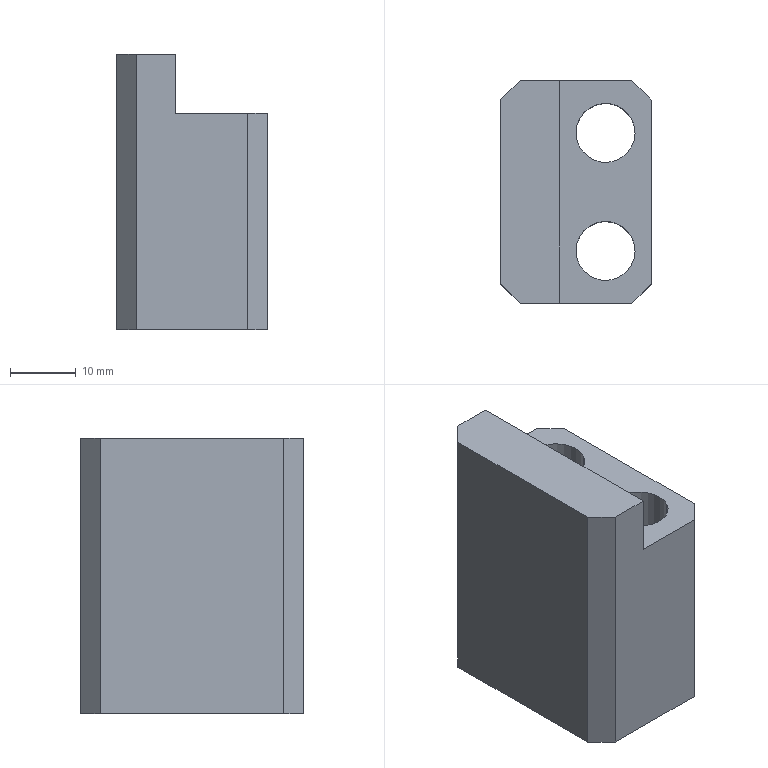Part | CATIA | 1 solid | 16 faces | box 23 x 34 x 42 mm | volume 23686 mm3 | plane 12 | cylinder 4 | commonest cylinder face diameters 9 x4
STEP:
#1=CARTESIAN_POINT('',(-1248.,-1169.,-42.));
#2=VERTEX_POINT('',#1);
#3=CARTESIAN_POINT('',(-1245.,-1172.,-42.));
#4=VERTEX_POINT('',#3);
#5=CARTESIAN_POINT('',(-1246.5,-1170.5,-42.));
#6=DIRECTION('',(0.7071,-0.7071,0.));
#7=VECTOR('',#6,1.);
#8=LINE('',#5,#7);
#9=EDGE_CURVE('',#2,#4,#8,.T.);
#10=ORIENTED_EDGE('',*,*,#9,.T.);
#11=CARTESIAN_POINT('',(-1245.,-1172.,0.));
#12=VERTEX_POINT('',#11);
#13=CARTESIAN_POINT('',(-1245.,-1172.,-21.));
#14=DIRECTION('',(0.,0.,-1.));
#15=VECTOR('',#14,1.);
#16=LINE('',#13,#15);
#17=EDGE_CURVE('',#12,#4,#16,.T.);
#18=ORIENTED_EDGE('',*,*,#17,.F.);
#19=CARTESIAN_POINT('',(-1248.,-1169.,0.));
#20=VERTEX_POINT('',#19);
#21=CARTESIAN_POINT('',(-1246.5,-1170.5,0.));
#22=DIRECTION('',(0.7071,-0.7071,0.));
#23=VECTOR('',#22,1.);
#24=LINE('',#21,#23);
#25=EDGE_CURVE('',#12,#20,#24,.F.);
#26=ORIENTED_EDGE('',*,*,#25,.T.);
#27=CARTESIAN_POINT('',(-1248.,-1169.,-21.));
#28=DIRECTION('',(0.,0.,-1.));
#29=VECTOR('',#28,1.);
#30=LINE('',#27,#29);
#31=EDGE_CURVE('',#20,#2,#30,.T.);
#32=ORIENTED_EDGE('',*,*,#31,.T.);
#33=EDGE_LOOP('',(#10,#18,#26,#32));
#34=FACE_OUTER_BOUND('',#33,.T.);
#35=CARTESIAN_POINT('',(-1248.,-1169.,8.4));
#36=DIRECTION('',(-0.7071,-0.7071,0.));
#37=DIRECTION('',(0.,0.,-1.));
#38=AXIS2_PLACEMENT_3D('',#35,#36,#37);
#39=PLANE('',#38);
#40=ADVANCED_FACE('',(#34),#39,.T.);
#41=CARTESIAN_POINT('',(-1248.,-1141.,0.));
#42=VERTEX_POINT('',#41);
#43=CARTESIAN_POINT('',(-1248.,-1141.,-42.));
#44=VERTEX_POINT('',#43);
#45=CARTESIAN_POINT('',(-1248.,-1141.,-21.));
#46=DIRECTION('',(0.,0.,1.));
#47=VECTOR('',#46,1.);
#48=LINE('',#45,#47);
#49=EDGE_CURVE('',#42,#44,#48,.F.);
#50=ORIENTED_EDGE('',*,*,#49,.T.);
#51=CARTESIAN_POINT('',(-1248.,-1155.,-42.));
#52=DIRECTION('',(0.,-1.,0.));
#53=VECTOR('',#52,1.);
#54=LINE('',#51,#53);
#55=EDGE_CURVE('',#44,#2,#54,.T.);
#56=ORIENTED_EDGE('',*,*,#55,.T.);
#57=ORIENTED_EDGE('',*,*,#31,.F.);
#58=CARTESIAN_POINT('',(-1248.,-1155.,0.));
#59=DIRECTION('',(0.,-1.,0.));
#60=VECTOR('',#59,1.);
#61=LINE('',#58,#60);
#62=EDGE_CURVE('',#42,#20,#61,.T.);
#63=ORIENTED_EDGE('',*,*,#62,.F.);
#64=EDGE_LOOP('',(#50,#56,#57,#63));
#65=FACE_OUTER_BOUND('',#64,.T.);
#66=CARTESIAN_POINT('',(-1248.,-1138.,0.));
#67=DIRECTION('',(1.,0.,0.));
#68=DIRECTION('',(0.,-1.,0.));
#69=AXIS2_PLACEMENT_3D('',#66,#67,#68);
#70=PLANE('',#69);
#71=ADVANCED_FACE('',(#65),#70,.F.);
#72=CARTESIAN_POINT('',(-1245.,-1138.,-42.));
#73=VERTEX_POINT('',#72);
#74=CARTESIAN_POINT('',(-1246.5,-1139.5,-42.));
#75=DIRECTION('',(0.7071,0.7071,0.));
#76=VECTOR('',#75,1.);
#77=LINE('',#74,#76);
#78=EDGE_CURVE('',#73,#44,#77,.F.);
#79=ORIENTED_EDGE('',*,*,#78,.T.);
#80=ORIENTED_EDGE('',*,*,#49,.F.);
#81=CARTESIAN_POINT('',(-1245.,-1138.,0.));
#82=VERTEX_POINT('',#81);
#83=CARTESIAN_POINT('',(-1246.5,-1139.5,0.));
#84=DIRECTION('',(0.7071,0.7071,0.));
#85=VECTOR('',#84,1.);
#86=LINE('',#83,#85);
#87=EDGE_CURVE('',#42,#82,#86,.T.);
#88=ORIENTED_EDGE('',*,*,#87,.T.);
#89=CARTESIAN_POINT('',(-1245.,-1138.,-21.));
#90=DIRECTION('',(0.,0.,1.));
#91=VECTOR('',#90,1.);
#92=LINE('',#89,#91);
#93=EDGE_CURVE('',#82,#73,#92,.F.);
#94=ORIENTED_EDGE('',*,*,#93,.T.);
#95=EDGE_LOOP('',(#79,#80,#88,#94));
#96=FACE_OUTER_BOUND('',#95,.T.);
#97=CARTESIAN_POINT('',(-1248.,-1141.,-50.4));
#98=DIRECTION('',(-0.7071,0.7071,0.));
#99=DIRECTION('',(0.,0.,1.));
#100=AXIS2_PLACEMENT_3D('',#97,#98,#99);
#101=PLANE('',#100);
#102=ADVANCED_FACE('',(#96),#101,.T.);
#103=CARTESIAN_POINT('',(-1225.,-1141.,-9.));
#104=VERTEX_POINT('',#103);
#105=CARTESIAN_POINT('',(-1225.,-1141.,-42.));
#106=VERTEX_POINT('',#105);
#107=CARTESIAN_POINT('',(-1225.,-1141.,-21.));
#108=DIRECTION('',(0.,0.,-1.));
#109=VECTOR('',#108,1.);
#110=LINE('',#107,#109);
#111=EDGE_CURVE('',#104,#106,#110,.T.);
#112=ORIENTED_EDGE('',*,*,#111,.T.);
#113=CARTESIAN_POINT('',(-1228.,-1138.,-42.));
#114=VERTEX_POINT('',#113);
#115=CARTESIAN_POINT('',(-1226.5,-1139.5,-42.));
#116=DIRECTION('',(-0.7071,0.7071,0.));
#117=VECTOR('',#116,1.);
#118=LINE('',#115,#117);
#119=EDGE_CURVE('',#106,#114,#118,.T.);
#120=ORIENTED_EDGE('',*,*,#119,.T.);
#121=CARTESIAN_POINT('',(-1228.,-1138.,-9.));
#122=VERTEX_POINT('',#121);
#123=CARTESIAN_POINT('',(-1228.,-1138.,-21.));
#124=DIRECTION('',(0.,0.,-1.));
#125=VECTOR('',#124,1.);
#126=LINE('',#123,#125);
#127=EDGE_CURVE('',#122,#114,#126,.T.);
#128=ORIENTED_EDGE('',*,*,#127,.F.);
#129=CARTESIAN_POINT('',(-1226.5,-1139.5,-9.));
#130=DIRECTION('',(-0.7071,0.7071,0.));
#131=VECTOR('',#130,1.);
#132=LINE('',#129,#131);
#133=EDGE_CURVE('',#122,#104,#132,.F.);
#134=ORIENTED_EDGE('',*,*,#133,.T.);
#135=EDGE_LOOP('',(#112,#120,#128,#134));
#136=FACE_OUTER_BOUND('',#135,.T.);
#137=CARTESIAN_POINT('',(-1225.,-1141.,8.4));
#138=DIRECTION('',(0.7071,0.7071,0.));
#139=DIRECTION('',(0.,0.,-1.));
#140=AXIS2_PLACEMENT_3D('',#137,#138,#139);
#141=PLANE('',#140);
#142=ADVANCED_FACE('',(#136),#141,.T.);
#143=CARTESIAN_POINT('',(-1239.,-1138.,0.));
#144=VERTEX_POINT('',#143);
#145=CARTESIAN_POINT('',(-1242.,-1138.,0.));
#146=DIRECTION('',(1.,0.,0.));
#147=VECTOR('',#146,1.);
#148=LINE('',#145,#147);
#149=EDGE_CURVE('',#144,#82,#148,.F.);
#150=ORIENTED_EDGE('',*,*,#149,.T.);
#151=ORIENTED_EDGE('',*,*,#87,.F.);
#152=ORIENTED_EDGE('',*,*,#62,.T.);
#153=ORIENTED_EDGE('',*,*,#25,.F.);
#154=CARTESIAN_POINT('',(-1239.,-1172.,0.));
#155=VERTEX_POINT('',#154);
#156=CARTESIAN_POINT('',(-1242.,-1172.,0.));
#157=DIRECTION('',(-1.,0.,0.));
#158=VECTOR('',#157,1.);
#159=LINE('',#156,#158);
#160=EDGE_CURVE('',#12,#155,#159,.F.);
#161=ORIENTED_EDGE('',*,*,#160,.T.);
#162=CARTESIAN_POINT('',(-1239.,-1155.,0.));
#163=DIRECTION('',(0.,-1.,0.));
#164=VECTOR('',#163,1.);
#165=LINE('',#162,#164);
#166=EDGE_CURVE('',#144,#155,#165,.T.);
#167=ORIENTED_EDGE('',*,*,#166,.F.);
#168=EDGE_LOOP('',(#150,#151,#152,#153,#161,#167));
#169=FACE_OUTER_BOUND('',#168,.T.);
#170=CARTESIAN_POINT('',(0.,0.,0.));
#171=DIRECTION('',(0.,0.,1.));
#172=DIRECTION('',(1.,0.,0.));
#173=AXIS2_PLACEMENT_3D('',#170,#171,#172);
#174=PLANE('',#173);
#175=ADVANCED_FACE('',(#169),#174,.T.);
#176=CARTESIAN_POINT('',(-1225.,-1169.,-9.));
#177=VERTEX_POINT('',#176);
#178=CARTESIAN_POINT('',(-1225.,-1155.,-9.));
#179=DIRECTION('',(0.,1.,0.));
#180=VECTOR('',#179,1.);
#181=LINE('',#178,#180);
#182=EDGE_CURVE('',#177,#104,#181,.T.);
#183=ORIENTED_EDGE('',*,*,#182,.F.);
#184=CARTESIAN_POINT('',(-1225.,-1169.,-42.));
#185=VERTEX_POINT('',#184);
#186=CARTESIAN_POINT('',(-1225.,-1169.,-25.5));
#187=DIRECTION('',(0.,0.,1.));
#188=VECTOR('',#187,1.);
#189=LINE('',#186,#188);
#190=EDGE_CURVE('',#177,#185,#189,.F.);
#191=ORIENTED_EDGE('',*,*,#190,.T.);
#192=CARTESIAN_POINT('',(-1225.,-1155.,-42.));
#193=DIRECTION('',(0.,1.,0.));
#194=VECTOR('',#193,1.);
#195=LINE('',#192,#194);
#196=EDGE_CURVE('',#185,#106,#195,.T.);
#197=ORIENTED_EDGE('',*,*,#196,.T.);
#198=ORIENTED_EDGE('',*,*,#111,.F.);
#199=EDGE_LOOP('',(#183,#191,#197,#198));
#200=FACE_OUTER_BOUND('',#199,.T.);
#201=CARTESIAN_POINT('',(-1225.,-1172.,0.));
#202=DIRECTION('',(-1.,0.,0.));
#203=DIRECTION('',(0.,1.,0.));
#204=AXIS2_PLACEMENT_3D('',#201,#202,#203);
#205=PLANE('',#204);
#206=ADVANCED_FACE('',(#200),#205,.F.);
#207=ORIENTED_EDGE('',*,*,#127,.T.);
#208=CARTESIAN_POINT('',(-1236.5,-1138.,-42.));
#209=DIRECTION('',(1.,0.,0.));
#210=VECTOR('',#209,1.);
#211=LINE('',#208,#210);
#212=EDGE_CURVE('',#73,#114,#211,.T.);
#213=ORIENTED_EDGE('',*,*,#212,.F.);
#214=ORIENTED_EDGE('',*,*,#93,.F.);
#215=ORIENTED_EDGE('',*,*,#149,.F.);
#216=CARTESIAN_POINT('',(-1239.,-1138.,-9.));
#217=VERTEX_POINT('',#216);
#218=CARTESIAN_POINT('',(-1239.,-1138.,-4.5));
#219=DIRECTION('',(0.,0.,1.));
#220=VECTOR('',#219,1.);
#221=LINE('',#218,#220);
#222=EDGE_CURVE('',#217,#144,#221,.T.);
#223=ORIENTED_EDGE('',*,*,#222,.F.);
#224=CARTESIAN_POINT('',(-1233.5,-1138.,-9.));
#225=DIRECTION('',(1.,0.,0.));
#226=VECTOR('',#225,1.);
#227=LINE('',#224,#226);
#228=EDGE_CURVE('',#217,#122,#227,.T.);
#229=ORIENTED_EDGE('',*,*,#228,.T.);
#230=EDGE_LOOP('',(#207,#213,#214,#215,#223,#229));
#231=FACE_OUTER_BOUND('',#230,.T.);
#232=CARTESIAN_POINT('',(-1248.,-1138.,0.));
#233=DIRECTION('',(0.,1.,0.));
#234=DIRECTION('',(1.,0.,0.));
#235=AXIS2_PLACEMENT_3D('',#232,#233,#234);
#236=PLANE('',#235);
#237=ADVANCED_FACE('',(#231),#236,.T.);
#238=CARTESIAN_POINT('',(-1228.,-1172.,-9.));
#239=VERTEX_POINT('',#238);
#240=CARTESIAN_POINT('',(-1228.,-1172.,-42.));
#241=VERTEX_POINT('',#240);
#242=CARTESIAN_POINT('',(-1228.,-1172.,-21.));
#243=DIRECTION('',(0.,0.,1.));
#244=VECTOR('',#243,1.);
#245=LINE('',#242,#244);
#246=EDGE_CURVE('',#239,#241,#245,.F.);
#247=ORIENTED_EDGE('',*,*,#246,.T.);
#248=CARTESIAN_POINT('',(-1226.5,-1170.5,-42.));
#249=DIRECTION('',(-0.7071,-0.7071,0.));
#250=VECTOR('',#249,1.);
#251=LINE('',#248,#250);
#252=EDGE_CURVE('',#241,#185,#251,.F.);
#253=ORIENTED_EDGE('',*,*,#252,.T.);
#254=ORIENTED_EDGE('',*,*,#190,.F.);
#255=CARTESIAN_POINT('',(-1226.5,-1170.5,-9.));
#256=DIRECTION('',(-0.7071,-0.7071,0.));
#257=VECTOR('',#256,1.);
#258=LINE('',#255,#257);
#259=EDGE_CURVE('',#239,#177,#258,.F.);
#260=ORIENTED_EDGE('',*,*,#259,.F.);
#261=EDGE_LOOP('',(#247,#253,#254,#260));
#262=FACE_OUTER_BOUND('',#261,.T.);
#263=CARTESIAN_POINT('',(-1225.,-1169.,-50.4));
#264=DIRECTION('',(0.7071,-0.7071,0.));
#265=DIRECTION('',(0.,0.,1.));
#266=AXIS2_PLACEMENT_3D('',#263,#264,#265);
#267=PLANE('',#266);
#268=ADVANCED_FACE('',(#262),#267,.T.);
#269=ORIENTED_EDGE('',*,*,#160,.F.);
#270=ORIENTED_EDGE('',*,*,#17,.T.);
#271=CARTESIAN_POINT('',(-1236.5,-1172.,-42.));
#272=DIRECTION('',(-1.,0.,0.));
#273=VECTOR('',#272,1.);
#274=LINE('',#271,#273);
#275=EDGE_CURVE('',#241,#4,#274,.T.);
#276=ORIENTED_EDGE('',*,*,#275,.F.);
#277=ORIENTED_EDGE('',*,*,#246,.F.);
#278=CARTESIAN_POINT('',(-1239.,-1172.,-9.));
#279=VERTEX_POINT('',#278);
#280=CARTESIAN_POINT('',(-1233.5,-1172.,-9.));
#281=DIRECTION('',(1.,0.,0.));
#282=VECTOR('',#281,1.);
#283=LINE('',#280,#282);
#284=EDGE_CURVE('',#279,#239,#283,.T.);
#285=ORIENTED_EDGE('',*,*,#284,.F.);
#286=CARTESIAN_POINT('',(-1239.,-1172.,-4.5));
#287=DIRECTION('',(0.,0.,1.));
#288=VECTOR('',#287,1.);
#289=LINE('',#286,#288);
#290=EDGE_CURVE('',#279,#155,#289,.T.);
#291=ORIENTED_EDGE('',*,*,#290,.T.);
#292=EDGE_LOOP('',(#269,#270,#276,#277,#285,#291));
#293=FACE_OUTER_BOUND('',#292,.T.);
#294=CARTESIAN_POINT('',(-1225.,-1172.,0.));
#295=DIRECTION('',(0.,-1.,0.));
#296=DIRECTION('',(-1.,0.,0.));
#297=AXIS2_PLACEMENT_3D('',#294,#295,#296);
#298=PLANE('',#297);
#299=ADVANCED_FACE('',(#293),#298,.T.);
#300=CARTESIAN_POINT('',(-1239.,-1155.,-9.));
#301=DIRECTION('',(0.,-1.,0.));
#302=VECTOR('',#301,1.);
#303=LINE('',#300,#302);
#304=EDGE_CURVE('',#217,#279,#303,.T.);
#305=ORIENTED_EDGE('',*,*,#304,.F.);
#306=ORIENTED_EDGE('',*,*,#222,.T.);
#307=ORIENTED_EDGE('',*,*,#166,.T.);
#308=ORIENTED_EDGE('',*,*,#290,.F.);
#309=EDGE_LOOP('',(#305,#306,#307,#308));
#310=FACE_OUTER_BOUND('',#309,.T.);
#311=CARTESIAN_POINT('',(-1239.,-1122.,0.));
#312=DIRECTION('',(1.,0.,0.));
#313=DIRECTION('',(0.,-1.,0.));
#314=AXIS2_PLACEMENT_3D('',#311,#312,#313);
#315=PLANE('',#314);
#316=ADVANCED_FACE('',(#310),#315,.T.);
#317=ORIENTED_EDGE('',*,*,#304,.T.);
#318=ORIENTED_EDGE('',*,*,#284,.T.);
#319=ORIENTED_EDGE('',*,*,#259,.T.);
#320=ORIENTED_EDGE('',*,*,#182,.T.);
#321=ORIENTED_EDGE('',*,*,#133,.F.);
#322=ORIENTED_EDGE('',*,*,#228,.F.);
#323=EDGE_LOOP('',(#317,#318,#319,#320,#321,#322));
#324=FACE_OUTER_BOUND('',#323,.T.);
#325=CARTESIAN_POINT('',(-1235.949,-1161.843,-9.));
#326=VERTEX_POINT('',#325);
#327=CARTESIAN_POINT('',(-1228.051,-1166.157,-9.));
#328=VERTEX_POINT('',#327);
#329=CARTESIAN_POINT('',(-1232.,-1164.,-9.));
#330=DIRECTION('',(0.,0.,1.));
#331=AXIS2_PLACEMENT_3D('',#329,#330,$);
#332=CIRCLE('',#331,4.5);
#333=EDGE_CURVE('',#326,#328,#332,.T.);
#334=ORIENTED_EDGE('',*,*,#333,.F.);
#335=CARTESIAN_POINT('',(-1232.,-1164.,-9.));
#336=DIRECTION('',(0.,0.,1.));
#337=AXIS2_PLACEMENT_3D('',#335,#336,$);
#338=CIRCLE('',#337,4.5);
#339=EDGE_CURVE('',#328,#326,#338,.T.);
#340=ORIENTED_EDGE('',*,*,#339,.F.);
#341=EDGE_LOOP('',(#334,#340));
#342=FACE_BOUND('',#341,.T.);
#343=CARTESIAN_POINT('',(-1235.949,-1143.843,-9.));
#344=VERTEX_POINT('',#343);
#345=CARTESIAN_POINT('',(-1228.051,-1148.157,-9.));
#346=VERTEX_POINT('',#345);
#347=CARTESIAN_POINT('',(-1232.,-1146.,-9.));
#348=DIRECTION('',(0.,0.,1.));
#349=AXIS2_PLACEMENT_3D('',#347,#348,$);
#350=CIRCLE('',#349,4.5);
#351=EDGE_CURVE('',#344,#346,#350,.T.);
#352=ORIENTED_EDGE('',*,*,#351,.F.);
#353=CARTESIAN_POINT('',(-1232.,-1146.,-9.));
#354=DIRECTION('',(0.,0.,1.));
#355=AXIS2_PLACEMENT_3D('',#353,#354,$);
#356=CIRCLE('',#355,4.5);
#357=EDGE_CURVE('',#346,#344,#356,.T.);
#358=ORIENTED_EDGE('',*,*,#357,.F.);
#359=EDGE_LOOP('',(#352,#358));
#360=FACE_BOUND('',#359,.T.);
#361=CARTESIAN_POINT('',(0.,0.,-9.));
#362=DIRECTION('',(0.,0.,1.));
#363=DIRECTION('',(1.,0.,0.));
#364=AXIS2_PLACEMENT_3D('',#361,#362,#363);
#365=PLANE('',#364);
#366=ADVANCED_FACE('',(#324,#342,#360),#365,.T.);
#367=ORIENTED_EDGE('',*,*,#119,.F.);
#368=ORIENTED_EDGE('',*,*,#196,.F.);
#369=ORIENTED_EDGE('',*,*,#252,.F.);
#370=ORIENTED_EDGE('',*,*,#275,.T.);
#371=ORIENTED_EDGE('',*,*,#9,.F.);
#372=ORIENTED_EDGE('',*,*,#55,.F.);
#373=ORIENTED_EDGE('',*,*,#78,.F.);
#374=ORIENTED_EDGE('',*,*,#212,.T.);
#375=EDGE_LOOP('',(#367,#368,#369,#370,#371,#372,#373,#374));
#376=FACE_OUTER_BOUND('',#375,.T.);
#377=CARTESIAN_POINT('',(-1235.949,-1161.843,-42.));
#378=VERTEX_POINT('',#377);
#379=CARTESIAN_POINT('',(-1228.051,-1166.157,-42.));
#380=VERTEX_POINT('',#379);
#381=CARTESIAN_POINT('',(-1232.,-1164.,-42.));
#382=DIRECTION('',(0.,0.,1.));
#383=AXIS2_PLACEMENT_3D('',#381,#382,$);
#384=CIRCLE('',#383,4.5);
#385=EDGE_CURVE('',#378,#380,#384,.T.);
#386=ORIENTED_EDGE('',*,*,#385,.T.);
#387=CARTESIAN_POINT('',(-1232.,-1164.,-42.));
#388=DIRECTION('',(0.,0.,1.));
#389=AXIS2_PLACEMENT_3D('',#387,#388,$);
#390=CIRCLE('',#389,4.5);
#391=EDGE_CURVE('',#380,#378,#390,.T.);
#392=ORIENTED_EDGE('',*,*,#391,.T.);
#393=EDGE_LOOP('',(#386,#392));
#394=FACE_BOUND('',#393,.T.);
#395=CARTESIAN_POINT('',(-1235.949,-1143.843,-42.));
#396=VERTEX_POINT('',#395);
#397=CARTESIAN_POINT('',(-1228.051,-1148.157,-42.));
#398=VERTEX_POINT('',#397);
#399=CARTESIAN_POINT('',(-1232.,-1146.,-42.));
#400=DIRECTION('',(0.,0.,1.));
#401=AXIS2_PLACEMENT_3D('',#399,#400,$);
#402=CIRCLE('',#401,4.5);
#403=EDGE_CURVE('',#396,#398,#402,.T.);
#404=ORIENTED_EDGE('',*,*,#403,.T.);
#405=CARTESIAN_POINT('',(-1232.,-1146.,-42.));
#406=DIRECTION('',(0.,0.,1.));
#407=AXIS2_PLACEMENT_3D('',#405,#406,$);
#408=CIRCLE('',#407,4.5);
#409=EDGE_CURVE('',#398,#396,#408,.T.);
#410=ORIENTED_EDGE('',*,*,#409,.T.);
#411=EDGE_LOOP('',(#404,#410));
#412=FACE_BOUND('',#411,.T.);
#413=CARTESIAN_POINT('',(0.,0.,-42.));
#414=DIRECTION('',(0.,0.,1.));
#415=DIRECTION('',(1.,0.,0.));
#416=AXIS2_PLACEMENT_3D('',#413,#414,#415);
#417=PLANE('',#416);
#418=ADVANCED_FACE('',(#376,#394,#412),#417,.F.);
#419=ORIENTED_EDGE('',*,*,#357,.T.);
#420=CARTESIAN_POINT('',(-1235.949,-1143.843,-21.));
#421=DIRECTION('',(0.,0.,-1.));
#422=VECTOR('',#421,1.);
#423=LINE('',#420,#422);
#424=EDGE_CURVE('',#396,#344,#423,.F.);
#425=ORIENTED_EDGE('',*,*,#424,.F.);
#426=ORIENTED_EDGE('',*,*,#409,.F.);
#427=CARTESIAN_POINT('',(-1228.051,-1148.157,-21.));
#428=DIRECTION('',(0.,0.,-1.));
#429=VECTOR('',#428,1.);
#430=LINE('',#427,#429);
#431=EDGE_CURVE('',#398,#346,#430,.F.);
#432=ORIENTED_EDGE('',*,*,#431,.T.);
#433=EDGE_LOOP('',(#419,#425,#426,#432));
#434=FACE_OUTER_BOUND('',#433,.T.);
#435=CARTESIAN_POINT('',(-1232.,-1146.,-0.1));
#436=DIRECTION('',(0.,0.,-1.));
#437=DIRECTION('',(0.8776,-0.4794,0.));
#438=AXIS2_PLACEMENT_3D('',#435,#436,#437);
#439=CYLINDRICAL_SURFACE('',#438,4.5);
#440=ADVANCED_FACE('',(#434),#439,.F.);
#441=ORIENTED_EDGE('',*,*,#351,.T.);
#442=ORIENTED_EDGE('',*,*,#431,.F.);
#443=ORIENTED_EDGE('',*,*,#403,.F.);
#444=ORIENTED_EDGE('',*,*,#424,.T.);
#445=EDGE_LOOP('',(#441,#442,#443,#444));
#446=FACE_OUTER_BOUND('',#445,.T.);
#447=ADVANCED_FACE('',(#446),#439,.F.);
#448=ORIENTED_EDGE('',*,*,#339,.T.);
#449=CARTESIAN_POINT('',(-1235.949,-1161.843,-21.));
#450=DIRECTION('',(0.,0.,-1.));
#451=VECTOR('',#450,1.);
#452=LINE('',#449,#451);
#453=EDGE_CURVE('',#378,#326,#452,.F.);
#454=ORIENTED_EDGE('',*,*,#453,.F.);
#455=ORIENTED_EDGE('',*,*,#391,.F.);
#456=CARTESIAN_POINT('',(-1228.051,-1166.157,-21.));
#457=DIRECTION('',(0.,0.,-1.));
#458=VECTOR('',#457,1.);
#459=LINE('',#456,#458);
#460=EDGE_CURVE('',#380,#328,#459,.F.);
#461=ORIENTED_EDGE('',*,*,#460,.T.);
#462=EDGE_LOOP('',(#448,#454,#455,#461));
#463=FACE_OUTER_BOUND('',#462,.T.);
#464=CARTESIAN_POINT('',(-1232.,-1164.,-0.1));
#465=DIRECTION('',(0.,0.,-1.));
#466=DIRECTION('',(0.8776,-0.4794,0.));
#467=AXIS2_PLACEMENT_3D('',#464,#465,#466);
#468=CYLINDRICAL_SURFACE('',#467,4.5);
#469=ADVANCED_FACE('',(#463),#468,.F.);
#470=ORIENTED_EDGE('',*,*,#333,.T.);
#471=ORIENTED_EDGE('',*,*,#460,.F.);
#472=ORIENTED_EDGE('',*,*,#385,.F.);
#473=ORIENTED_EDGE('',*,*,#453,.T.);
#474=EDGE_LOOP('',(#470,#471,#472,#473));
#475=FACE_OUTER_BOUND('',#474,.T.);
#476=ADVANCED_FACE('',(#475),#468,.F.);
#477=CLOSED_SHELL('',(#40,#71,#102,#142,#175,#206,#237,#268,#299,#316,#366,#418,#440,#447,#469,#476));
#478=MANIFOLD_SOLID_BREP('',#477);
#479=(LENGTH_UNIT()NAMED_UNIT(*)SI_UNIT(.MILLI.,.METRE.));
#480=UNCERTAINTY_MEASURE_WITH_UNIT(LENGTH_MEASURE(0.005),#479,'','');
#481=(NAMED_UNIT(*)PLANE_ANGLE_UNIT()SI_UNIT($,.RADIAN.));
#482=(NAMED_UNIT(*)SI_UNIT($,.STERADIAN.)SOLID_ANGLE_UNIT());
#483=(GEOMETRIC_REPRESENTATION_CONTEXT(3)GLOBAL_UNCERTAINTY_ASSIGNED_CONTEXT((#480))GLOBAL_UNIT_ASSIGNED_CONTEXT((#479,#481,#482))REPRESENTATION_CONTEXT('',''));
#484=ADVANCED_BREP_SHAPE_REPRESENTATION('',(#478),#483);